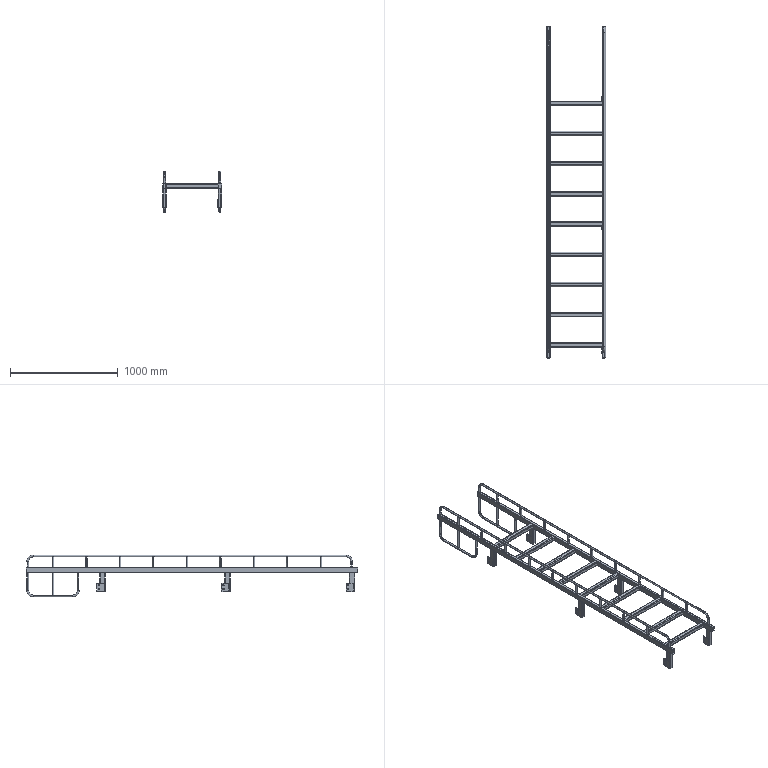Part | STEP file | 49 solids | 618 faces | box 548 x 3075 x 388 mm | volume 6786009 mm3 | cylinder 308 | plane 278 | spline 32 | commonest cylinder face diameters 18 x84 13 x64 8 x36 16 x36 5 x32 11 x32